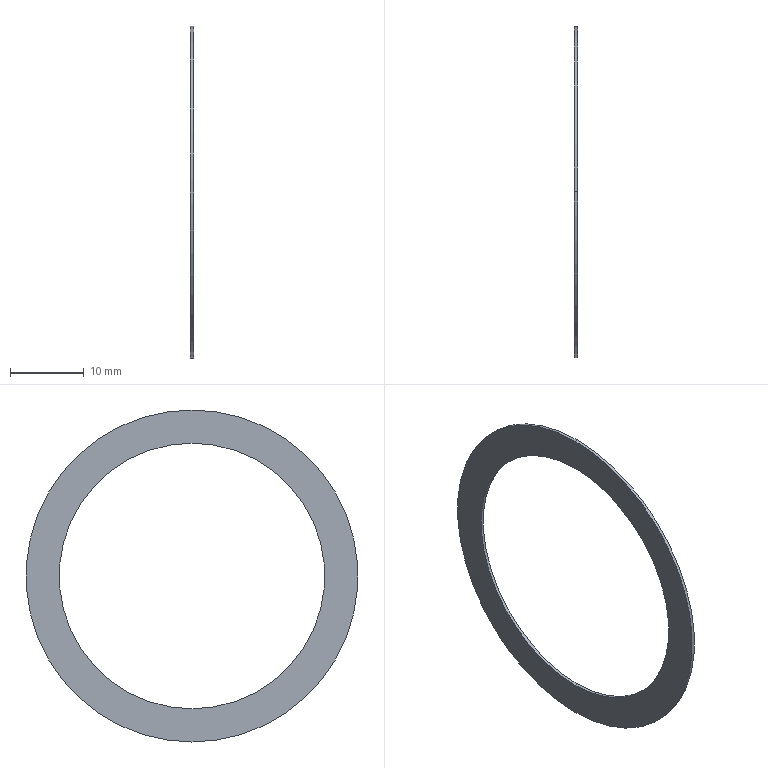Part | SolidWorks | features Extrusion 1 | 1 solid | 6 faces | box 0.41 x 45 x 45 mm | volume 234.748 mm3 | cylinder 4 | plane 2 | commonest cylinder face diameters 36 x2 45 x2
STEP:
#1=CARTESIAN_POINT('',(0.41,0.,18.));
#2=VERTEX_POINT('',#1);
#3=CARTESIAN_POINT('',(0.41,0.,-18.));
#4=VERTEX_POINT('',#3);
#5=CARTESIAN_POINT('',(0.41,0.,0.));
#6=DIRECTION('',(1.,0.,0.));
#7=DIRECTION('',(0.,0.,-1.));
#8=AXIS2_PLACEMENT_3D('',#5,#6,#7);
#9=CIRCLE('',#8,18.);
#10=EDGE_CURVE('',#2,#4,#9,.T.);
#11=ORIENTED_EDGE('',*,*,#10,.T.);
#12=CARTESIAN_POINT('',(0.,0.,-18.));
#13=VERTEX_POINT('',#12);
#14=CARTESIAN_POINT('',(0.41,0.,-18.));
#15=DIRECTION('',(-1.,0.,0.));
#16=VECTOR('',#15,1000.);
#17=LINE('',#14,#16);
#18=EDGE_CURVE('',#4,#13,#17,.T.);
#19=ORIENTED_EDGE('',*,*,#18,.T.);
#20=CARTESIAN_POINT('',(0.,0.,18.));
#21=VERTEX_POINT('',#20);
#22=CARTESIAN_POINT('',(0.,0.,0.));
#23=DIRECTION('',(1.,0.,0.));
#24=DIRECTION('',(0.,0.,-1.));
#25=AXIS2_PLACEMENT_3D('',#22,#23,#24);
#26=CIRCLE('',#25,18.);
#27=EDGE_CURVE('',#21,#13,#26,.T.);
#28=ORIENTED_EDGE('',*,*,#27,.F.);
#29=CARTESIAN_POINT('',(0.41,0.,18.));
#30=DIRECTION('',(-1.,0.,0.));
#31=VECTOR('',#30,1000.);
#32=LINE('',#29,#31);
#33=EDGE_CURVE('',#2,#21,#32,.T.);
#34=ORIENTED_EDGE('',*,*,#33,.F.);
#35=EDGE_LOOP('',(#11,#19,#28,#34));
#36=FACE_OUTER_BOUND('',#35,.T.);
#37=CARTESIAN_POINT('',(0.41,0.,0.));
#38=DIRECTION('',(-1.,0.,0.));
#39=DIRECTION('',(0.,0.,1.));
#40=AXIS2_PLACEMENT_3D('',#37,#38,#39);
#41=CYLINDRICAL_SURFACE('',#40,18.);
#42=ADVANCED_FACE('',(#36),#41,.F.);
#43=CARTESIAN_POINT('',(0.41,0.,-22.5));
#44=VERTEX_POINT('',#43);
#45=CARTESIAN_POINT('',(0.41,0.,22.5));
#46=VERTEX_POINT('',#45);
#47=CARTESIAN_POINT('',(0.41,0.,0.));
#48=DIRECTION('',(1.,0.,0.));
#49=DIRECTION('',(0.,0.,-1.));
#50=AXIS2_PLACEMENT_3D('',#47,#48,#49);
#51=CIRCLE('',#50,22.5);
#52=EDGE_CURVE('',#44,#46,#51,.T.);
#53=ORIENTED_EDGE('',*,*,#52,.F.);
#54=CARTESIAN_POINT('',(0.,0.,-22.5));
#55=VERTEX_POINT('',#54);
#56=CARTESIAN_POINT('',(0.41,0.,-22.5));
#57=DIRECTION('',(-1.,0.,0.));
#58=VECTOR('',#57,1000.);
#59=LINE('',#56,#58);
#60=EDGE_CURVE('',#44,#55,#59,.T.);
#61=ORIENTED_EDGE('',*,*,#60,.T.);
#62=CARTESIAN_POINT('',(0.,0.,22.5));
#63=VERTEX_POINT('',#62);
#64=CARTESIAN_POINT('',(0.,0.,0.));
#65=DIRECTION('',(1.,0.,0.));
#66=DIRECTION('',(0.,0.,-1.));
#67=AXIS2_PLACEMENT_3D('',#64,#65,#66);
#68=CIRCLE('',#67,22.5);
#69=EDGE_CURVE('',#55,#63,#68,.T.);
#70=ORIENTED_EDGE('',*,*,#69,.T.);
#71=CARTESIAN_POINT('',(0.41,0.,22.5));
#72=DIRECTION('',(-1.,0.,0.));
#73=VECTOR('',#72,1000.);
#74=LINE('',#71,#73);
#75=EDGE_CURVE('',#46,#63,#74,.T.);
#76=ORIENTED_EDGE('',*,*,#75,.F.);
#77=EDGE_LOOP('',(#53,#61,#70,#76));
#78=FACE_OUTER_BOUND('',#77,.T.);
#79=CARTESIAN_POINT('',(0.41,0.,0.));
#80=DIRECTION('',(-1.,0.,0.));
#81=DIRECTION('',(0.,0.,1.));
#82=AXIS2_PLACEMENT_3D('',#79,#80,#81);
#83=CYLINDRICAL_SURFACE('',#82,22.5);
#84=ADVANCED_FACE('',(#78),#83,.T.);
#85=CARTESIAN_POINT('',(0.41,0.,0.));
#86=DIRECTION('',(1.,0.,0.));
#87=DIRECTION('',(0.,0.,-1.));
#88=AXIS2_PLACEMENT_3D('',#85,#86,#87);
#89=CIRCLE('',#88,22.5);
#90=EDGE_CURVE('',#46,#44,#89,.T.);
#91=ORIENTED_EDGE('',*,*,#90,.T.);
#92=ORIENTED_EDGE('',*,*,#52,.T.);
#93=EDGE_LOOP('',(#91,#92));
#94=FACE_OUTER_BOUND('',#93,.T.);
#95=ORIENTED_EDGE('',*,*,#10,.F.);
#96=CARTESIAN_POINT('',(0.41,0.,0.));
#97=DIRECTION('',(1.,0.,0.));
#98=DIRECTION('',(0.,0.,-1.));
#99=AXIS2_PLACEMENT_3D('',#96,#97,#98);
#100=CIRCLE('',#99,18.);
#101=EDGE_CURVE('',#4,#2,#100,.T.);
#102=ORIENTED_EDGE('',*,*,#101,.F.);
#103=EDGE_LOOP('',(#95,#102));
#104=FACE_BOUND('',#103,.T.);
#105=CARTESIAN_POINT('',(0.41,0.,0.));
#106=DIRECTION('',(1.,0.,0.));
#107=DIRECTION('',(0.,0.,-1.));
#108=AXIS2_PLACEMENT_3D('',#105,#106,#107);
#109=PLANE('',#108);
#110=ADVANCED_FACE('',(#94,#104),#109,.T.);
#111=CARTESIAN_POINT('',(0.,0.,0.));
#112=DIRECTION('',(1.,0.,0.));
#113=DIRECTION('',(0.,0.,-1.));
#114=AXIS2_PLACEMENT_3D('',#111,#112,#113);
#115=CIRCLE('',#114,22.5);
#116=EDGE_CURVE('',#63,#55,#115,.T.);
#117=ORIENTED_EDGE('',*,*,#116,.F.);
#118=ORIENTED_EDGE('',*,*,#69,.F.);
#119=EDGE_LOOP('',(#117,#118));
#120=FACE_OUTER_BOUND('',#119,.T.);
#121=ORIENTED_EDGE('',*,*,#27,.T.);
#122=CARTESIAN_POINT('',(0.,0.,0.));
#123=DIRECTION('',(1.,0.,0.));
#124=DIRECTION('',(0.,0.,-1.));
#125=AXIS2_PLACEMENT_3D('',#122,#123,#124);
#126=CIRCLE('',#125,18.);
#127=EDGE_CURVE('',#13,#21,#126,.T.);
#128=ORIENTED_EDGE('',*,*,#127,.T.);
#129=EDGE_LOOP('',(#121,#128));
#130=FACE_BOUND('',#129,.T.);
#131=CARTESIAN_POINT('',(0.,0.,0.));
#132=DIRECTION('',(1.,0.,0.));
#133=DIRECTION('',(0.,0.,-1.));
#134=AXIS2_PLACEMENT_3D('',#131,#132,#133);
#135=PLANE('',#134);
#136=ADVANCED_FACE('',(#120,#130),#135,.F.);
#137=ORIENTED_EDGE('',*,*,#60,.F.);
#138=ORIENTED_EDGE('',*,*,#90,.F.);
#139=ORIENTED_EDGE('',*,*,#75,.T.);
#140=ORIENTED_EDGE('',*,*,#116,.T.);
#141=EDGE_LOOP('',(#137,#138,#139,#140));
#142=FACE_OUTER_BOUND('',#141,.T.);
#143=CARTESIAN_POINT('',(0.41,0.,0.));
#144=DIRECTION('',(-1.,0.,0.));
#145=DIRECTION('',(0.,0.,1.));
#146=AXIS2_PLACEMENT_3D('',#143,#144,#145);
#147=CYLINDRICAL_SURFACE('',#146,22.5);
#148=ADVANCED_FACE('',(#142),#147,.T.);
#149=ORIENTED_EDGE('',*,*,#18,.F.);
#150=ORIENTED_EDGE('',*,*,#101,.T.);
#151=ORIENTED_EDGE('',*,*,#33,.T.);
#152=ORIENTED_EDGE('',*,*,#127,.F.);
#153=EDGE_LOOP('',(#149,#150,#151,#152));
#154=FACE_OUTER_BOUND('',#153,.T.);
#155=CARTESIAN_POINT('',(0.41,0.,0.));
#156=DIRECTION('',(-1.,0.,0.));
#157=DIRECTION('',(0.,0.,1.));
#158=AXIS2_PLACEMENT_3D('',#155,#156,#157);
#159=CYLINDRICAL_SURFACE('',#158,18.);
#160=ADVANCED_FACE('',(#154),#159,.F.);
#161=CLOSED_SHELL('',(#42,#84,#110,#136,#148,#160));
#162=MANIFOLD_SOLID_BREP('',#161);
#163=CARTESIAN_POINT('',(0.,0.,0.));
#164=DIRECTION('',(0.,0.,1.));
#165=DIRECTION('',(1.,0.,0.));
#166=AXIS2_PLACEMENT_3D('',#163,#164,#165);
#167=(LENGTH_UNIT()NAMED_UNIT(*)SI_UNIT(.MILLI.,.METRE.));
#168=UNCERTAINTY_MEASURE_WITH_UNIT(LENGTH_MEASURE(0.00001),#167,'','');
#169=(NAMED_UNIT(*)PLANE_ANGLE_UNIT()SI_UNIT($,.RADIAN.));
#170=(NAMED_UNIT(*)SI_UNIT($,.STERADIAN.)SOLID_ANGLE_UNIT());
#171=(GEOMETRIC_REPRESENTATION_CONTEXT(3)GLOBAL_UNCERTAINTY_ASSIGNED_CONTEXT((#168))GLOBAL_UNIT_ASSIGNED_CONTEXT((#167,#169,#170))REPRESENTATION_CONTEXT('',''));
#172=ADVANCED_BREP_SHAPE_REPRESENTATION('',(#162,#166),#171);